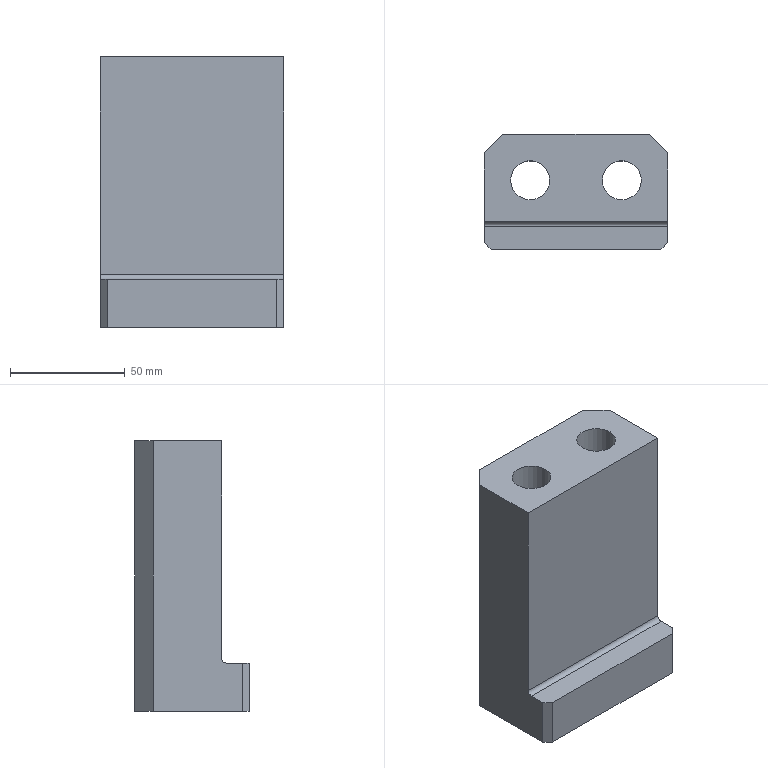Part | STEP file | PN_0041_id1270_x_t | 1 solid | 19 faces | box 80 x 50 x 118 mm | volume 264145 mm3 | plane 14 | cylinder 5 | commonest cylinder face diameters 17 x2 26 x2 4 x1
STEP:
#1=CARTESIAN_POINT('',(-313.5,218.5,105.));
#2=VERTEX_POINT('',#1);
#3=CARTESIAN_POINT('',(-305.,218.5,105.));
#4=DIRECTION('',(0.,0.,-1.));
#5=DIRECTION('',(-1.,0.,0.));
#6=AXIS2_PLACEMENT_3D('',#3,#4,#5);
#7=CIRCLE('',#6,8.5);
#8=EDGE_CURVE('',#2,#2,#7,.T.);
#9=ORIENTED_EDGE('',*,*,#8,.T.);
#10=EDGE_LOOP('',(#9));
#11=FACE_BOUND('',#10,.T.);
#12=CARTESIAN_POINT('',(-353.5,218.5,105.));
#13=VERTEX_POINT('',#12);
#14=CARTESIAN_POINT('',(-345.,218.5,105.));
#15=DIRECTION('',(0.,0.,-1.));
#16=DIRECTION('',(-1.,0.,0.));
#17=AXIS2_PLACEMENT_3D('',#14,#15,#16);
#18=CIRCLE('',#17,8.5);
#19=EDGE_CURVE('',#13,#13,#18,.T.);
#20=ORIENTED_EDGE('',*,*,#19,.T.);
#21=EDGE_LOOP('',(#20));
#22=FACE_BOUND('',#21,.T.);
#23=CARTESIAN_POINT('',(-285.,230.5,105.));
#24=VERTEX_POINT('',#23);
#25=CARTESIAN_POINT('',(-285.,200.5,105.));
#26=VERTEX_POINT('',#25);
#27=CARTESIAN_POINT('',(-285.,238.,105.));
#28=DIRECTION('',(0.,-1.,0.));
#29=VECTOR('',#28,1.);
#30=LINE('',#27,#29);
#31=EDGE_CURVE('',#24,#26,#30,.T.);
#32=ORIENTED_EDGE('',*,*,#31,.F.);
#33=CARTESIAN_POINT('',(-293.,238.5,105.));
#34=VERTEX_POINT('',#33);
#35=CARTESIAN_POINT('',(-305.,250.5,105.));
#36=DIRECTION('',(-0.7071,0.7071,0.));
#37=VECTOR('',#36,1.);
#38=LINE('',#35,#37);
#39=EDGE_CURVE('',#24,#34,#38,.T.);
#40=ORIENTED_EDGE('',*,*,#39,.T.);
#41=CARTESIAN_POINT('',(-357.,238.5,105.));
#42=VERTEX_POINT('',#41);
#43=CARTESIAN_POINT('',(-317.5,238.5,105.));
#44=DIRECTION('',(1.,0.,0.));
#45=VECTOR('',#44,1.);
#46=LINE('',#43,#45);
#47=EDGE_CURVE('',#42,#34,#46,.T.);
#48=ORIENTED_EDGE('',*,*,#47,.F.);
#49=CARTESIAN_POINT('',(-365.,230.5,105.));
#50=VERTEX_POINT('',#49);
#51=CARTESIAN_POINT('',(-337.5,258.,105.));
#52=DIRECTION('',(-0.7071,-0.7071,0.));
#53=VECTOR('',#52,1.);
#54=LINE('',#51,#53);
#55=EDGE_CURVE('',#42,#50,#54,.T.);
#56=ORIENTED_EDGE('',*,*,#55,.T.);
#57=CARTESIAN_POINT('',(-365.,200.5,105.));
#58=VERTEX_POINT('',#57);
#59=CARTESIAN_POINT('',(-365.,238.,105.));
#60=DIRECTION('',(0.,1.,0.));
#61=VECTOR('',#60,1.);
#62=LINE('',#59,#61);
#63=EDGE_CURVE('',#58,#50,#62,.T.);
#64=ORIENTED_EDGE('',*,*,#63,.F.);
#65=CARTESIAN_POINT('',(-317.5,200.5,105.));
#66=DIRECTION('',(1.,0.,0.));
#67=VECTOR('',#66,1.);
#68=LINE('',#65,#67);
#69=EDGE_CURVE('',#58,#26,#68,.T.);
#70=ORIENTED_EDGE('',*,*,#69,.T.);
#71=EDGE_LOOP('',(#32,#40,#48,#56,#64,#70));
#72=FACE_BOUND('',#71,.T.);
#73=CARTESIAN_POINT('',(-317.5,238.,105.));
#74=DIRECTION('',(0.,0.,1.));
#75=DIRECTION('',(-1.,0.,0.));
#76=AXIS2_PLACEMENT_3D('',#73,#74,#75);
#77=PLANE('',#76);
#78=ADVANCED_FACE('',(#11,#22,#72),#77,.T.);
#79=CARTESIAN_POINT('',(-285.,191.5,-13.));
#80=VERTEX_POINT('',#79);
#81=CARTESIAN_POINT('',(-285.,230.5,-13.));
#82=VERTEX_POINT('',#81);
#83=CARTESIAN_POINT('',(-285.,238.,-13.));
#84=DIRECTION('',(0.,1.,0.));
#85=VECTOR('',#84,1.);
#86=LINE('',#83,#85);
#87=EDGE_CURVE('',#80,#82,#86,.T.);
#88=ORIENTED_EDGE('',*,*,#87,.T.);
#89=CARTESIAN_POINT('',(-285.,230.5,-88.));
#90=DIRECTION('',(0.,0.,1.));
#91=VECTOR('',#90,1.);
#92=LINE('',#89,#91);
#93=EDGE_CURVE('',#82,#24,#92,.T.);
#94=ORIENTED_EDGE('',*,*,#93,.T.);
#95=ORIENTED_EDGE('',*,*,#31,.T.);
#96=CARTESIAN_POINT('',(-285.,200.5,10.));
#97=VERTEX_POINT('',#96);
#98=CARTESIAN_POINT('',(-285.,200.5,-76.));
#99=DIRECTION('',(0.,0.,1.));
#100=VECTOR('',#99,1.);
#101=LINE('',#98,#100);
#102=EDGE_CURVE('',#97,#26,#101,.T.);
#103=ORIENTED_EDGE('',*,*,#102,.F.);
#104=CARTESIAN_POINT('',(-285.,198.5,8.));
#105=VERTEX_POINT('',#104);
#106=CARTESIAN_POINT('',(-285.,198.5,10.));
#107=DIRECTION('',(-1.,0.,0.));
#108=DIRECTION('',(0.,0.,1.));
#109=AXIS2_PLACEMENT_3D('',#106,#107,#108);
#110=CIRCLE('',#109,2.);
#111=EDGE_CURVE('',#97,#105,#110,.T.);
#112=ORIENTED_EDGE('',*,*,#111,.T.);
#113=CARTESIAN_POINT('',(-285.,191.5,8.));
#114=VERTEX_POINT('',#113);
#115=CARTESIAN_POINT('',(-285.,195.5,8.));
#116=DIRECTION('',(0.,1.,0.));
#117=VECTOR('',#116,1.);
#118=LINE('',#115,#117);
#119=EDGE_CURVE('',#114,#105,#118,.T.);
#120=ORIENTED_EDGE('',*,*,#119,.F.);
#121=CARTESIAN_POINT('',(-285.,191.5,-8.));
#122=DIRECTION('',(0.,0.,-1.));
#123=VECTOR('',#122,1.);
#124=LINE('',#121,#123);
#125=EDGE_CURVE('',#114,#80,#124,.T.);
#126=ORIENTED_EDGE('',*,*,#125,.T.);
#127=EDGE_LOOP('',(#88,#94,#95,#103,#112,#120,#126));
#128=FACE_OUTER_BOUND('',#127,.T.);
#129=CARTESIAN_POINT('',(-285.,238.,-88.));
#130=DIRECTION('',(1.,0.,0.));
#131=DIRECTION('',(0.,0.,1.));
#132=AXIS2_PLACEMENT_3D('',#129,#130,#131);
#133=PLANE('',#132);
#134=ADVANCED_FACE('',(#128),#133,.T.);
#135=CARTESIAN_POINT('',(-362.,188.5,-13.));
#136=VERTEX_POINT('',#135);
#137=CARTESIAN_POINT('',(-288.,188.5,-13.));
#138=VERTEX_POINT('',#137);
#139=CARTESIAN_POINT('',(-317.5,188.5,-13.));
#140=DIRECTION('',(1.,0.,0.));
#141=VECTOR('',#140,1.);
#142=LINE('',#139,#141);
#143=EDGE_CURVE('',#136,#138,#142,.T.);
#144=ORIENTED_EDGE('',*,*,#143,.T.);
#145=CARTESIAN_POINT('',(-288.,188.5,8.));
#146=VERTEX_POINT('',#145);
#147=CARTESIAN_POINT('',(-288.,188.5,-8.));
#148=DIRECTION('',(0.,0.,1.));
#149=VECTOR('',#148,1.);
#150=LINE('',#147,#149);
#151=EDGE_CURVE('',#138,#146,#150,.T.);
#152=ORIENTED_EDGE('',*,*,#151,.T.);
#153=CARTESIAN_POINT('',(-362.,188.5,8.));
#154=VERTEX_POINT('',#153);
#155=CARTESIAN_POINT('',(-317.5,188.5,8.));
#156=DIRECTION('',(1.,0.,0.));
#157=VECTOR('',#156,1.);
#158=LINE('',#155,#157);
#159=EDGE_CURVE('',#154,#146,#158,.T.);
#160=ORIENTED_EDGE('',*,*,#159,.F.);
#161=CARTESIAN_POINT('',(-362.,188.5,-8.));
#162=DIRECTION('',(0.,0.,-1.));
#163=VECTOR('',#162,1.);
#164=LINE('',#161,#163);
#165=EDGE_CURVE('',#154,#136,#164,.T.);
#166=ORIENTED_EDGE('',*,*,#165,.T.);
#167=EDGE_LOOP('',(#144,#152,#160,#166));
#168=FACE_OUTER_BOUND('',#167,.T.);
#169=CARTESIAN_POINT('',(-317.5,188.5,-8.));
#170=DIRECTION('',(0.,-1.,0.));
#171=DIRECTION('',(0.,0.,1.));
#172=AXIS2_PLACEMENT_3D('',#169,#170,#171);
#173=PLANE('',#172);
#174=ADVANCED_FACE('',(#168),#173,.T.);
#175=CARTESIAN_POINT('',(-318.,218.5,-13.));
#176=VERTEX_POINT('',#175);
#177=CARTESIAN_POINT('',(-305.,218.5,-13.));
#178=DIRECTION('',(0.,0.,1.));
#179=DIRECTION('',(-1.,0.,0.));
#180=AXIS2_PLACEMENT_3D('',#177,#178,#179);
#181=CIRCLE('',#180,13.);
#182=EDGE_CURVE('',#176,#176,#181,.T.);
#183=ORIENTED_EDGE('',*,*,#182,.T.);
#184=EDGE_LOOP('',(#183));
#185=FACE_BOUND('',#184,.T.);
#186=CARTESIAN_POINT('',(-358.,218.5,-13.));
#187=VERTEX_POINT('',#186);
#188=CARTESIAN_POINT('',(-345.,218.5,-13.));
#189=DIRECTION('',(0.,0.,1.));
#190=DIRECTION('',(-1.,0.,0.));
#191=AXIS2_PLACEMENT_3D('',#188,#189,#190);
#192=CIRCLE('',#191,13.);
#193=EDGE_CURVE('',#187,#187,#192,.T.);
#194=ORIENTED_EDGE('',*,*,#193,.T.);
#195=EDGE_LOOP('',(#194));
#196=FACE_BOUND('',#195,.T.);
#197=CARTESIAN_POINT('',(-293.,238.5,-13.));
#198=VERTEX_POINT('',#197);
#199=CARTESIAN_POINT('',(-357.,238.5,-13.));
#200=VERTEX_POINT('',#199);
#201=CARTESIAN_POINT('',(-317.5,238.5,-13.));
#202=DIRECTION('',(-1.,0.,0.));
#203=VECTOR('',#202,1.);
#204=LINE('',#201,#203);
#205=EDGE_CURVE('',#198,#200,#204,.T.);
#206=ORIENTED_EDGE('',*,*,#205,.F.);
#207=CARTESIAN_POINT('',(-305.,250.5,-13.));
#208=DIRECTION('',(0.7071,-0.7071,0.));
#209=VECTOR('',#208,1.);
#210=LINE('',#207,#209);
#211=EDGE_CURVE('',#198,#82,#210,.T.);
#212=ORIENTED_EDGE('',*,*,#211,.T.);
#213=ORIENTED_EDGE('',*,*,#87,.F.);
#214=CARTESIAN_POINT('',(-274.,202.5,-13.));
#215=DIRECTION('',(-0.7071,-0.7071,0.));
#216=VECTOR('',#215,1.);
#217=LINE('',#214,#216);
#218=EDGE_CURVE('',#80,#138,#217,.T.);
#219=ORIENTED_EDGE('',*,*,#218,.T.);
#220=ORIENTED_EDGE('',*,*,#143,.F.);
#221=CARTESIAN_POINT('',(-365.,191.5,-13.));
#222=VERTEX_POINT('',#221);
#223=CARTESIAN_POINT('',(-366.,192.5,-13.));
#224=DIRECTION('',(-0.7071,0.7071,0.));
#225=VECTOR('',#224,1.);
#226=LINE('',#223,#225);
#227=EDGE_CURVE('',#136,#222,#226,.T.);
#228=ORIENTED_EDGE('',*,*,#227,.T.);
#229=CARTESIAN_POINT('',(-365.,230.5,-13.));
#230=VERTEX_POINT('',#229);
#231=CARTESIAN_POINT('',(-365.,238.,-13.));
#232=DIRECTION('',(0.,-1.,0.));
#233=VECTOR('',#232,1.);
#234=LINE('',#231,#233);
#235=EDGE_CURVE('',#230,#222,#234,.T.);
#236=ORIENTED_EDGE('',*,*,#235,.F.);
#237=CARTESIAN_POINT('',(-337.5,258.,-13.));
#238=DIRECTION('',(0.7071,0.7071,0.));
#239=VECTOR('',#238,1.);
#240=LINE('',#237,#239);
#241=EDGE_CURVE('',#230,#200,#240,.T.);
#242=ORIENTED_EDGE('',*,*,#241,.T.);
#243=EDGE_LOOP('',(#206,#212,#213,#219,#220,#228,#236,#242));
#244=FACE_BOUND('',#243,.T.);
#245=CARTESIAN_POINT('',(-317.5,238.,-13.));
#246=DIRECTION('',(0.,0.,-1.));
#247=DIRECTION('',(1.,0.,0.));
#248=AXIS2_PLACEMENT_3D('',#245,#246,#247);
#249=PLANE('',#248);
#250=ADVANCED_FACE('',(#185,#196,#244),#249,.T.);
#251=ORIENTED_EDGE('',*,*,#63,.T.);
#252=CARTESIAN_POINT('',(-365.,230.5,-88.));
#253=DIRECTION('',(0.,0.,-1.));
#254=VECTOR('',#253,1.);
#255=LINE('',#252,#254);
#256=EDGE_CURVE('',#50,#230,#255,.T.);
#257=ORIENTED_EDGE('',*,*,#256,.T.);
#258=ORIENTED_EDGE('',*,*,#235,.T.);
#259=CARTESIAN_POINT('',(-365.,191.5,8.));
#260=VERTEX_POINT('',#259);
#261=CARTESIAN_POINT('',(-365.,191.5,-8.));
#262=DIRECTION('',(0.,0.,1.));
#263=VECTOR('',#262,1.);
#264=LINE('',#261,#263);
#265=EDGE_CURVE('',#222,#260,#264,.T.);
#266=ORIENTED_EDGE('',*,*,#265,.T.);
#267=CARTESIAN_POINT('',(-365.,198.5,8.));
#268=VERTEX_POINT('',#267);
#269=CARTESIAN_POINT('',(-365.,195.5,8.));
#270=DIRECTION('',(0.,-1.,0.));
#271=VECTOR('',#270,1.);
#272=LINE('',#269,#271);
#273=EDGE_CURVE('',#268,#260,#272,.T.);
#274=ORIENTED_EDGE('',*,*,#273,.F.);
#275=CARTESIAN_POINT('',(-365.,200.5,10.));
#276=VERTEX_POINT('',#275);
#277=CARTESIAN_POINT('',(-365.,198.5,10.));
#278=DIRECTION('',(1.,0.,0.));
#279=DIRECTION('',(0.,0.,-1.));
#280=AXIS2_PLACEMENT_3D('',#277,#278,#279);
#281=CIRCLE('',#280,2.);
#282=EDGE_CURVE('',#268,#276,#281,.T.);
#283=ORIENTED_EDGE('',*,*,#282,.T.);
#284=CARTESIAN_POINT('',(-365.,200.5,-76.));
#285=DIRECTION('',(0.,0.,1.));
#286=VECTOR('',#285,1.);
#287=LINE('',#284,#286);
#288=EDGE_CURVE('',#276,#58,#287,.T.);
#289=ORIENTED_EDGE('',*,*,#288,.T.);
#290=EDGE_LOOP('',(#251,#257,#258,#266,#274,#283,#289));
#291=FACE_OUTER_BOUND('',#290,.T.);
#292=CARTESIAN_POINT('',(-365.,238.,-88.));
#293=DIRECTION('',(-1.,0.,0.));
#294=DIRECTION('',(0.,0.,-1.));
#295=AXIS2_PLACEMENT_3D('',#292,#293,#294);
#296=PLANE('',#295);
#297=ADVANCED_FACE('',(#291),#296,.T.);
#298=ORIENTED_EDGE('',*,*,#288,.F.);
#299=CARTESIAN_POINT('',(-317.5,200.5,10.));
#300=DIRECTION('',(1.,0.,0.));
#301=VECTOR('',#300,1.);
#302=LINE('',#299,#301);
#303=EDGE_CURVE('',#276,#97,#302,.T.);
#304=ORIENTED_EDGE('',*,*,#303,.T.);
#305=ORIENTED_EDGE('',*,*,#102,.T.);
#306=ORIENTED_EDGE('',*,*,#69,.F.);
#307=EDGE_LOOP('',(#298,#304,#305,#306));
#308=FACE_OUTER_BOUND('',#307,.T.);
#309=CARTESIAN_POINT('',(-317.5,200.5,-76.));
#310=DIRECTION('',(0.,1.,0.));
#311=DIRECTION('',(0.,0.,-1.));
#312=AXIS2_PLACEMENT_3D('',#309,#310,#311);
#313=PLANE('',#312);
#314=ADVANCED_FACE('',(#308),#313,.F.);
#315=ORIENTED_EDGE('',*,*,#119,.T.);
#316=CARTESIAN_POINT('',(-340.,198.5,8.));
#317=DIRECTION('',(-1.,0.,0.));
#318=VECTOR('',#317,1.);
#319=LINE('',#316,#318);
#320=EDGE_CURVE('',#105,#268,#319,.T.);
#321=ORIENTED_EDGE('',*,*,#320,.T.);
#322=ORIENTED_EDGE('',*,*,#273,.T.);
#323=CARTESIAN_POINT('',(-365.,191.5,8.));
#324=DIRECTION('',(0.7071,-0.7071,0.));
#325=VECTOR('',#324,1.);
#326=LINE('',#323,#325);
#327=EDGE_CURVE('',#260,#154,#326,.T.);
#328=ORIENTED_EDGE('',*,*,#327,.T.);
#329=ORIENTED_EDGE('',*,*,#159,.T.);
#330=CARTESIAN_POINT('',(-288.,188.5,8.));
#331=DIRECTION('',(0.7071,0.7071,0.));
#332=VECTOR('',#331,1.);
#333=LINE('',#330,#332);
#334=EDGE_CURVE('',#146,#114,#333,.T.);
#335=ORIENTED_EDGE('',*,*,#334,.T.);
#336=EDGE_LOOP('',(#315,#321,#322,#328,#329,#335));
#337=FACE_OUTER_BOUND('',#336,.T.);
#338=CARTESIAN_POINT('',(-317.5,195.5,8.));
#339=DIRECTION('',(0.,0.,-1.));
#340=DIRECTION('',(1.,0.,0.));
#341=AXIS2_PLACEMENT_3D('',#338,#339,#340);
#342=PLANE('',#341);
#343=ADVANCED_FACE('',(#337),#342,.F.);
#344=ORIENTED_EDGE('',*,*,#218,.F.);
#345=ORIENTED_EDGE('',*,*,#125,.F.);
#346=ORIENTED_EDGE('',*,*,#334,.F.);
#347=ORIENTED_EDGE('',*,*,#151,.F.);
#348=EDGE_LOOP('',(#344,#345,#346,#347));
#349=FACE_OUTER_BOUND('',#348,.T.);
#350=CARTESIAN_POINT('',(-288.,188.5,-8.));
#351=DIRECTION('',(-0.7071,0.7071,0.));
#352=DIRECTION('',(-0.7071,-0.7071,0.));
#353=AXIS2_PLACEMENT_3D('',#350,#351,#352);
#354=PLANE('',#353);
#355=ADVANCED_FACE('',(#349),#354,.F.);
#356=ORIENTED_EDGE('',*,*,#227,.F.);
#357=ORIENTED_EDGE('',*,*,#165,.F.);
#358=ORIENTED_EDGE('',*,*,#327,.F.);
#359=ORIENTED_EDGE('',*,*,#265,.F.);
#360=EDGE_LOOP('',(#356,#357,#358,#359));
#361=FACE_OUTER_BOUND('',#360,.T.);
#362=CARTESIAN_POINT('',(-365.,191.5,-8.));
#363=DIRECTION('',(0.7071,0.7071,0.));
#364=DIRECTION('',(-0.7071,0.7071,0.));
#365=AXIS2_PLACEMENT_3D('',#362,#363,#364);
#366=PLANE('',#365);
#367=ADVANCED_FACE('',(#361),#366,.F.);
#368=ORIENTED_EDGE('',*,*,#111,.F.);
#369=ORIENTED_EDGE('',*,*,#303,.F.);
#370=ORIENTED_EDGE('',*,*,#282,.F.);
#371=ORIENTED_EDGE('',*,*,#320,.F.);
#372=EDGE_LOOP('',(#368,#369,#370,#371));
#373=FACE_OUTER_BOUND('',#372,.T.);
#374=CARTESIAN_POINT('',(-317.5,198.5,10.));
#375=DIRECTION('',(1.,0.,0.));
#376=DIRECTION('',(0.,0.,1.));
#377=AXIS2_PLACEMENT_3D('',#374,#375,#376);
#378=CYLINDRICAL_SURFACE('',#377,2.);
#379=ADVANCED_FACE('',(#373),#378,.F.);
#380=ORIENTED_EDGE('',*,*,#47,.T.);
#381=CARTESIAN_POINT('',(-293.,238.5,-88.));
#382=DIRECTION('',(0.,0.,-1.));
#383=VECTOR('',#382,1.);
#384=LINE('',#381,#383);
#385=EDGE_CURVE('',#34,#198,#384,.T.);
#386=ORIENTED_EDGE('',*,*,#385,.T.);
#387=ORIENTED_EDGE('',*,*,#205,.T.);
#388=CARTESIAN_POINT('',(-357.,238.5,-88.));
#389=DIRECTION('',(0.,0.,1.));
#390=VECTOR('',#389,1.);
#391=LINE('',#388,#390);
#392=EDGE_CURVE('',#200,#42,#391,.T.);
#393=ORIENTED_EDGE('',*,*,#392,.T.);
#394=EDGE_LOOP('',(#380,#386,#387,#393));
#395=FACE_OUTER_BOUND('',#394,.T.);
#396=CARTESIAN_POINT('',(-317.5,238.5,-88.));
#397=DIRECTION('',(0.,1.,0.));
#398=DIRECTION('',(0.,0.,-1.));
#399=AXIS2_PLACEMENT_3D('',#396,#397,#398);
#400=PLANE('',#399);
#401=ADVANCED_FACE('',(#395),#400,.T.);
#402=ORIENTED_EDGE('',*,*,#39,.F.);
#403=ORIENTED_EDGE('',*,*,#93,.F.);
#404=ORIENTED_EDGE('',*,*,#211,.F.);
#405=ORIENTED_EDGE('',*,*,#385,.F.);
#406=EDGE_LOOP('',(#402,#403,#404,#405));
#407=FACE_OUTER_BOUND('',#406,.T.);
#408=CARTESIAN_POINT('',(-293.,238.5,-88.));
#409=DIRECTION('',(-0.7071,-0.7071,0.));
#410=DIRECTION('',(0.,0.,-1.));
#411=AXIS2_PLACEMENT_3D('',#408,#409,#410);
#412=PLANE('',#411);
#413=ADVANCED_FACE('',(#407),#412,.F.);
#414=ORIENTED_EDGE('',*,*,#55,.F.);
#415=ORIENTED_EDGE('',*,*,#392,.F.);
#416=ORIENTED_EDGE('',*,*,#241,.F.);
#417=ORIENTED_EDGE('',*,*,#256,.F.);
#418=EDGE_LOOP('',(#414,#415,#416,#417));
#419=FACE_OUTER_BOUND('',#418,.T.);
#420=CARTESIAN_POINT('',(-365.,230.5,-88.));
#421=DIRECTION('',(0.7071,-0.7071,0.));
#422=DIRECTION('',(0.,0.,-1.));
#423=AXIS2_PLACEMENT_3D('',#420,#421,#422);
#424=PLANE('',#423);
#425=ADVANCED_FACE('',(#419),#424,.F.);
#426=CARTESIAN_POINT('',(-336.5,218.5,75.));
#427=VERTEX_POINT('',#426);
#428=CARTESIAN_POINT('',(-345.,218.5,75.));
#429=DIRECTION('',(0.,0.,1.));
#430=DIRECTION('',(1.,0.,0.));
#431=AXIS2_PLACEMENT_3D('',#428,#429,#430);
#432=CIRCLE('',#431,8.5);
#433=EDGE_CURVE('',#427,#427,#432,.T.);
#434=ORIENTED_EDGE('',*,*,#433,.F.);
#435=EDGE_LOOP('',(#434));
#436=FACE_BOUND('',#435,.T.);
#437=ORIENTED_EDGE('',*,*,#19,.F.);
#438=EDGE_LOOP('',(#437));
#439=FACE_BOUND('',#438,.T.);
#440=CARTESIAN_POINT('',(-345.,218.5,105.));
#441=DIRECTION('',(0.,0.,-1.));
#442=DIRECTION('',(-1.,0.,0.));
#443=AXIS2_PLACEMENT_3D('',#440,#441,#442);
#444=CYLINDRICAL_SURFACE('',#443,8.5);
#445=ADVANCED_FACE('',(#436,#439),#444,.F.);
#446=ORIENTED_EDGE('',*,*,#433,.T.);
#447=EDGE_LOOP('',(#446));
#448=FACE_BOUND('',#447,.T.);
#449=CARTESIAN_POINT('',(-358.,218.5,75.));
#450=VERTEX_POINT('',#449);
#451=CARTESIAN_POINT('',(-345.,218.5,75.));
#452=DIRECTION('',(0.,0.,1.));
#453=DIRECTION('',(-1.,0.,0.));
#454=AXIS2_PLACEMENT_3D('',#451,#452,#453);
#455=CIRCLE('',#454,13.);
#456=EDGE_CURVE('',#450,#450,#455,.T.);
#457=ORIENTED_EDGE('',*,*,#456,.F.);
#458=EDGE_LOOP('',(#457));
#459=FACE_BOUND('',#458,.T.);
#460=CARTESIAN_POINT('',(-345.,218.5,75.));
#461=DIRECTION('',(0.,0.,1.));
#462=DIRECTION('',(1.,0.,0.));
#463=AXIS2_PLACEMENT_3D('',#460,#461,#462);
#464=PLANE('',#463);
#465=ADVANCED_FACE('',(#448,#459),#464,.F.);
#466=ORIENTED_EDGE('',*,*,#193,.F.);
#467=EDGE_LOOP('',(#466));
#468=FACE_BOUND('',#467,.T.);
#469=ORIENTED_EDGE('',*,*,#456,.T.);
#470=EDGE_LOOP('',(#469));
#471=FACE_BOUND('',#470,.T.);
#472=CARTESIAN_POINT('',(-345.,218.5,75.));
#473=DIRECTION('',(0.,0.,-1.));
#474=DIRECTION('',(-1.,0.,0.));
#475=AXIS2_PLACEMENT_3D('',#472,#473,#474);
#476=CYLINDRICAL_SURFACE('',#475,13.);
#477=ADVANCED_FACE('',(#468,#471),#476,.F.);
#478=CARTESIAN_POINT('',(-296.5,218.5,75.));
#479=VERTEX_POINT('',#478);
#480=CARTESIAN_POINT('',(-305.,218.5,75.));
#481=DIRECTION('',(0.,0.,1.));
#482=DIRECTION('',(1.,0.,0.));
#483=AXIS2_PLACEMENT_3D('',#480,#481,#482);
#484=CIRCLE('',#483,8.5);
#485=EDGE_CURVE('',#479,#479,#484,.T.);
#486=ORIENTED_EDGE('',*,*,#485,.F.);
#487=EDGE_LOOP('',(#486));
#488=FACE_BOUND('',#487,.T.);
#489=ORIENTED_EDGE('',*,*,#8,.F.);
#490=EDGE_LOOP('',(#489));
#491=FACE_BOUND('',#490,.T.);
#492=CARTESIAN_POINT('',(-305.,218.5,105.));
#493=DIRECTION('',(0.,0.,-1.));
#494=DIRECTION('',(-1.,0.,0.));
#495=AXIS2_PLACEMENT_3D('',#492,#493,#494);
#496=CYLINDRICAL_SURFACE('',#495,8.5);
#497=ADVANCED_FACE('',(#488,#491),#496,.F.);
#498=ORIENTED_EDGE('',*,*,#485,.T.);
#499=EDGE_LOOP('',(#498));
#500=FACE_BOUND('',#499,.T.);
#501=CARTESIAN_POINT('',(-318.,218.5,75.));
#502=VERTEX_POINT('',#501);
#503=CARTESIAN_POINT('',(-305.,218.5,75.));
#504=DIRECTION('',(0.,0.,1.));
#505=DIRECTION('',(-1.,0.,0.));
#506=AXIS2_PLACEMENT_3D('',#503,#504,#505);
#507=CIRCLE('',#506,13.);
#508=EDGE_CURVE('',#502,#502,#507,.T.);
#509=ORIENTED_EDGE('',*,*,#508,.F.);
#510=EDGE_LOOP('',(#509));
#511=FACE_BOUND('',#510,.T.);
#512=CARTESIAN_POINT('',(-305.,218.5,75.));
#513=DIRECTION('',(0.,0.,1.));
#514=DIRECTION('',(1.,0.,0.));
#515=AXIS2_PLACEMENT_3D('',#512,#513,#514);
#516=PLANE('',#515);
#517=ADVANCED_FACE('',(#500,#511),#516,.F.);
#518=ORIENTED_EDGE('',*,*,#182,.F.);
#519=EDGE_LOOP('',(#518));
#520=FACE_BOUND('',#519,.T.);
#521=ORIENTED_EDGE('',*,*,#508,.T.);
#522=EDGE_LOOP('',(#521));
#523=FACE_BOUND('',#522,.T.);
#524=CARTESIAN_POINT('',(-305.,218.5,75.));
#525=DIRECTION('',(0.,0.,-1.));
#526=DIRECTION('',(-1.,0.,0.));
#527=AXIS2_PLACEMENT_3D('',#524,#525,#526);
#528=CYLINDRICAL_SURFACE('',#527,13.);
#529=ADVANCED_FACE('',(#520,#523),#528,.F.);
#530=CLOSED_SHELL('',(#78,#134,#174,#250,#297,#314,#343,#355,#367,#379,#401,#413,#425,#445,#465,#477,#497,#517,#529));
#531=MANIFOLD_SOLID_BREP('',#530);
#532=(LENGTH_UNIT()NAMED_UNIT(*)SI_UNIT(.MILLI.,.METRE.));
#533=UNCERTAINTY_MEASURE_WITH_UNIT(LENGTH_MEASURE(0.00002),#532,'','');
#534=(NAMED_UNIT(*)PLANE_ANGLE_UNIT()SI_UNIT($,.RADIAN.));
#535=PLANE_ANGLE_MEASURE_WITH_UNIT(PLANE_ANGLE_MEASURE(0.01745),#534);
#536=DIMENSIONAL_EXPONENTS(0.,0.,0.,0.,0.,0.,0.);
#537=(CONVERSION_BASED_UNIT('DEGREE',#535)NAMED_UNIT(#536)PLANE_ANGLE_UNIT());
#538=(NAMED_UNIT(*)SI_UNIT($,.STERADIAN.)SOLID_ANGLE_UNIT());
#539=(GEOMETRIC_REPRESENTATION_CONTEXT(3)GLOBAL_UNCERTAINTY_ASSIGNED_CONTEXT((#533))GLOBAL_UNIT_ASSIGNED_CONTEXT((#532,#537,#538))REPRESENTATION_CONTEXT('',''));
#540=ADVANCED_BREP_SHAPE_REPRESENTATION('',(#531),#539);